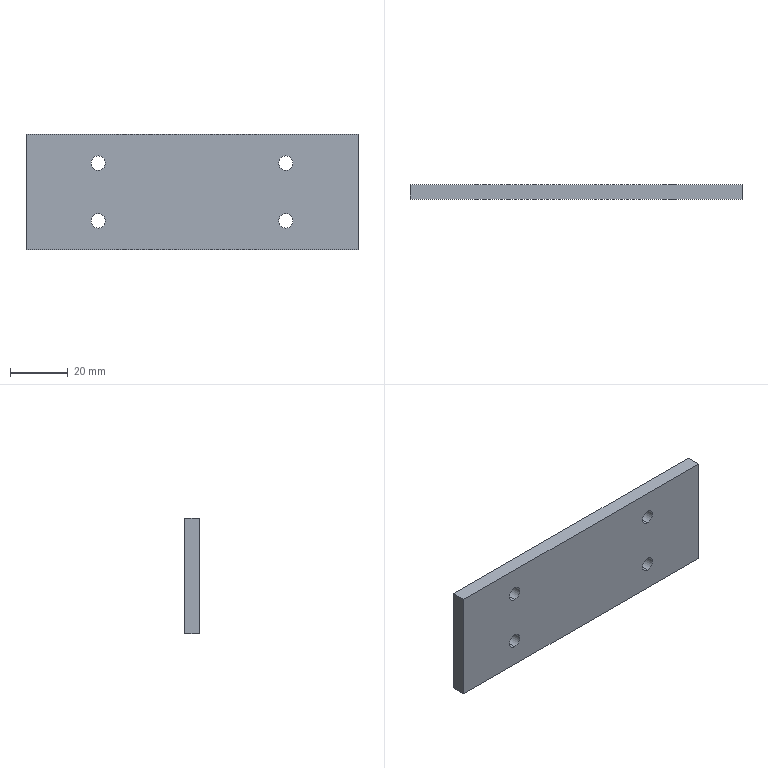Part | SolidWorks | features Extrusion 1, ICE 1 | 1 solid | 14 faces | box 115 x 5 x 40 mm | volume 22607 mm3 | cylinder 8 | plane 6 | commonest cylinder face diameters 5 x8
STEP:
#1=CARTESIAN_POINT('',(1.28,-0.09843,-0.2953));
#2=VERTEX_POINT('',#1);
#3=CARTESIAN_POINT('',(1.28,-0.09843,-0.4921));
#4=VERTEX_POINT('',#3);
#5=CARTESIAN_POINT('',(1.28,-0.09843,-0.3937));
#6=DIRECTION('',(0.,-1.,0.));
#7=DIRECTION('',(0.,0.,-1.));
#8=AXIS2_PLACEMENT_3D('',#5,#6,#7);
#9=CIRCLE('',#8,0.09843);
#10=EDGE_CURVE('',#2,#4,#9,.T.);
#11=ORIENTED_EDGE('',*,*,#10,.T.);
#12=CARTESIAN_POINT('',(1.28,0.09843,-0.4921));
#13=VERTEX_POINT('',#12);
#14=CARTESIAN_POINT('',(1.28,-1.476,-0.4921));
#15=DIRECTION('',(0.,1.,0.));
#16=VECTOR('',#15,39.37);
#17=LINE('',#14,#16);
#18=EDGE_CURVE('',#4,#13,#17,.T.);
#19=ORIENTED_EDGE('',*,*,#18,.T.);
#20=CARTESIAN_POINT('',(1.28,0.09843,-0.2953));
#21=VERTEX_POINT('',#20);
#22=CARTESIAN_POINT('',(1.28,0.09843,-0.3937));
#23=DIRECTION('',(0.,1.,0.));
#24=DIRECTION('',(0.,0.,1.));
#25=AXIS2_PLACEMENT_3D('',#22,#23,#24);
#26=CIRCLE('',#25,0.09843);
#27=EDGE_CURVE('',#13,#21,#26,.T.);
#28=ORIENTED_EDGE('',*,*,#27,.T.);
#29=CARTESIAN_POINT('',(1.28,-1.476,-0.2953));
#30=DIRECTION('',(0.,1.,0.));
#31=VECTOR('',#30,39.37);
#32=LINE('',#29,#31);
#33=EDGE_CURVE('',#2,#21,#32,.T.);
#34=ORIENTED_EDGE('',*,*,#33,.F.);
#35=EDGE_LOOP('',(#11,#19,#28,#34));
#36=FACE_OUTER_BOUND('',#35,.T.);
#37=CARTESIAN_POINT('',(1.28,-1.476,-0.3937));
#38=DIRECTION('',(0.,1.,0.));
#39=DIRECTION('',(0.,0.,1.));
#40=AXIS2_PLACEMENT_3D('',#37,#38,#39);
#41=CYLINDRICAL_SURFACE('',#40,0.09843);
#42=ADVANCED_FACE('',(#36),#41,.F.);
#43=CARTESIAN_POINT('',(-1.28,-0.09843,-0.2953));
#44=VERTEX_POINT('',#43);
#45=CARTESIAN_POINT('',(-1.28,-0.09843,-0.4921));
#46=VERTEX_POINT('',#45);
#47=CARTESIAN_POINT('',(-1.28,-0.09843,-0.3937));
#48=DIRECTION('',(0.,-1.,0.));
#49=DIRECTION('',(0.,0.,-1.));
#50=AXIS2_PLACEMENT_3D('',#47,#48,#49);
#51=CIRCLE('',#50,0.09843);
#52=EDGE_CURVE('',#44,#46,#51,.T.);
#53=ORIENTED_EDGE('',*,*,#52,.T.);
#54=CARTESIAN_POINT('',(-1.28,0.09843,-0.4921));
#55=VERTEX_POINT('',#54);
#56=CARTESIAN_POINT('',(-1.28,-1.476,-0.4921));
#57=DIRECTION('',(0.,1.,0.));
#58=VECTOR('',#57,39.37);
#59=LINE('',#56,#58);
#60=EDGE_CURVE('',#46,#55,#59,.T.);
#61=ORIENTED_EDGE('',*,*,#60,.T.);
#62=CARTESIAN_POINT('',(-1.28,0.09843,-0.2953));
#63=VERTEX_POINT('',#62);
#64=CARTESIAN_POINT('',(-1.28,0.09843,-0.3937));
#65=DIRECTION('',(0.,1.,0.));
#66=DIRECTION('',(0.,0.,1.));
#67=AXIS2_PLACEMENT_3D('',#64,#65,#66);
#68=CIRCLE('',#67,0.09843);
#69=EDGE_CURVE('',#55,#63,#68,.T.);
#70=ORIENTED_EDGE('',*,*,#69,.T.);
#71=CARTESIAN_POINT('',(-1.28,-1.476,-0.2953));
#72=DIRECTION('',(0.,1.,0.));
#73=VECTOR('',#72,39.37);
#74=LINE('',#71,#73);
#75=EDGE_CURVE('',#44,#63,#74,.T.);
#76=ORIENTED_EDGE('',*,*,#75,.F.);
#77=EDGE_LOOP('',(#53,#61,#70,#76));
#78=FACE_OUTER_BOUND('',#77,.T.);
#79=CARTESIAN_POINT('',(-1.28,-1.476,-0.3937));
#80=DIRECTION('',(0.,1.,0.));
#81=DIRECTION('',(0.,0.,1.));
#82=AXIS2_PLACEMENT_3D('',#79,#80,#81);
#83=CYLINDRICAL_SURFACE('',#82,0.09843);
#84=ADVANCED_FACE('',(#78),#83,.F.);
#85=CARTESIAN_POINT('',(1.28,-0.09843,-1.083));
#86=VERTEX_POINT('',#85);
#87=CARTESIAN_POINT('',(1.28,-0.09843,-1.28));
#88=VERTEX_POINT('',#87);
#89=CARTESIAN_POINT('',(1.28,-0.09843,-1.181));
#90=DIRECTION('',(0.,-1.,0.));
#91=DIRECTION('',(0.,0.,-1.));
#92=AXIS2_PLACEMENT_3D('',#89,#90,#91);
#93=CIRCLE('',#92,0.09843);
#94=EDGE_CURVE('',#86,#88,#93,.T.);
#95=ORIENTED_EDGE('',*,*,#94,.T.);
#96=CARTESIAN_POINT('',(1.28,0.09843,-1.28));
#97=VERTEX_POINT('',#96);
#98=CARTESIAN_POINT('',(1.28,-1.476,-1.28));
#99=DIRECTION('',(0.,1.,0.));
#100=VECTOR('',#99,39.37);
#101=LINE('',#98,#100);
#102=EDGE_CURVE('',#88,#97,#101,.T.);
#103=ORIENTED_EDGE('',*,*,#102,.T.);
#104=CARTESIAN_POINT('',(1.28,0.09843,-1.083));
#105=VERTEX_POINT('',#104);
#106=CARTESIAN_POINT('',(1.28,0.09843,-1.181));
#107=DIRECTION('',(0.,1.,0.));
#108=DIRECTION('',(0.,0.,1.));
#109=AXIS2_PLACEMENT_3D('',#106,#107,#108);
#110=CIRCLE('',#109,0.09843);
#111=EDGE_CURVE('',#97,#105,#110,.T.);
#112=ORIENTED_EDGE('',*,*,#111,.T.);
#113=CARTESIAN_POINT('',(1.28,-1.476,-1.083));
#114=DIRECTION('',(0.,1.,0.));
#115=VECTOR('',#114,39.37);
#116=LINE('',#113,#115);
#117=EDGE_CURVE('',#86,#105,#116,.T.);
#118=ORIENTED_EDGE('',*,*,#117,.F.);
#119=EDGE_LOOP('',(#95,#103,#112,#118));
#120=FACE_OUTER_BOUND('',#119,.T.);
#121=CARTESIAN_POINT('',(1.28,-1.476,-1.181));
#122=DIRECTION('',(0.,1.,0.));
#123=DIRECTION('',(0.,0.,1.));
#124=AXIS2_PLACEMENT_3D('',#121,#122,#123);
#125=CYLINDRICAL_SURFACE('',#124,0.09843);
#126=ADVANCED_FACE('',(#120),#125,.F.);
#127=CARTESIAN_POINT('',(-1.28,-0.09843,-1.083));
#128=VERTEX_POINT('',#127);
#129=CARTESIAN_POINT('',(-1.28,-0.09843,-1.28));
#130=VERTEX_POINT('',#129);
#131=CARTESIAN_POINT('',(-1.28,-0.09843,-1.181));
#132=DIRECTION('',(0.,-1.,0.));
#133=DIRECTION('',(0.,0.,-1.));
#134=AXIS2_PLACEMENT_3D('',#131,#132,#133);
#135=CIRCLE('',#134,0.09843);
#136=EDGE_CURVE('',#128,#130,#135,.T.);
#137=ORIENTED_EDGE('',*,*,#136,.T.);
#138=CARTESIAN_POINT('',(-1.28,0.09843,-1.28));
#139=VERTEX_POINT('',#138);
#140=CARTESIAN_POINT('',(-1.28,-1.476,-1.28));
#141=DIRECTION('',(0.,1.,0.));
#142=VECTOR('',#141,39.37);
#143=LINE('',#140,#142);
#144=EDGE_CURVE('',#130,#139,#143,.T.);
#145=ORIENTED_EDGE('',*,*,#144,.T.);
#146=CARTESIAN_POINT('',(-1.28,0.09843,-1.083));
#147=VERTEX_POINT('',#146);
#148=CARTESIAN_POINT('',(-1.28,0.09843,-1.181));
#149=DIRECTION('',(0.,1.,0.));
#150=DIRECTION('',(0.,0.,1.));
#151=AXIS2_PLACEMENT_3D('',#148,#149,#150);
#152=CIRCLE('',#151,0.09843);
#153=EDGE_CURVE('',#139,#147,#152,.T.);
#154=ORIENTED_EDGE('',*,*,#153,.T.);
#155=CARTESIAN_POINT('',(-1.28,-1.476,-1.083));
#156=DIRECTION('',(0.,1.,0.));
#157=VECTOR('',#156,39.37);
#158=LINE('',#155,#157);
#159=EDGE_CURVE('',#128,#147,#158,.T.);
#160=ORIENTED_EDGE('',*,*,#159,.F.);
#161=EDGE_LOOP('',(#137,#145,#154,#160));
#162=FACE_OUTER_BOUND('',#161,.T.);
#163=CARTESIAN_POINT('',(-1.28,-1.476,-1.181));
#164=DIRECTION('',(0.,1.,0.));
#165=DIRECTION('',(0.,0.,1.));
#166=AXIS2_PLACEMENT_3D('',#163,#164,#165);
#167=CYLINDRICAL_SURFACE('',#166,0.09843);
#168=ADVANCED_FACE('',(#162),#167,.F.);
#169=CARTESIAN_POINT('',(2.264,-0.09843,0.));
#170=VERTEX_POINT('',#169);
#171=CARTESIAN_POINT('',(2.264,0.09843,0.));
#172=VERTEX_POINT('',#171);
#173=CARTESIAN_POINT('',(2.264,0.09843,0.));
#174=DIRECTION('',(0.,1.,0.));
#175=VECTOR('',#174,39.37);
#176=LINE('',#173,#175);
#177=EDGE_CURVE('',#170,#172,#176,.T.);
#178=ORIENTED_EDGE('',*,*,#177,.F.);
#179=CARTESIAN_POINT('',(2.264,-0.09843,-1.575));
#180=VERTEX_POINT('',#179);
#181=CARTESIAN_POINT('',(2.264,-0.09843,-1.575));
#182=DIRECTION('',(0.,0.,1.));
#183=VECTOR('',#182,39.37);
#184=LINE('',#181,#183);
#185=EDGE_CURVE('',#180,#170,#184,.T.);
#186=ORIENTED_EDGE('',*,*,#185,.F.);
#187=CARTESIAN_POINT('',(2.264,0.09843,-1.575));
#188=VERTEX_POINT('',#187);
#189=CARTESIAN_POINT('',(2.264,0.09843,-1.575));
#190=DIRECTION('',(0.,1.,0.));
#191=VECTOR('',#190,39.37);
#192=LINE('',#189,#191);
#193=EDGE_CURVE('',#180,#188,#192,.T.);
#194=ORIENTED_EDGE('',*,*,#193,.T.);
#195=CARTESIAN_POINT('',(2.264,0.09843,-1.575));
#196=DIRECTION('',(0.,0.,1.));
#197=VECTOR('',#196,39.37);
#198=LINE('',#195,#197);
#199=EDGE_CURVE('',#188,#172,#198,.T.);
#200=ORIENTED_EDGE('',*,*,#199,.T.);
#201=EDGE_LOOP('',(#178,#186,#194,#200));
#202=FACE_OUTER_BOUND('',#201,.T.);
#203=CARTESIAN_POINT('',(2.264,0.09843,-1.575));
#204=DIRECTION('',(1.,0.,0.));
#205=DIRECTION('',(0.,0.,-1.));
#206=AXIS2_PLACEMENT_3D('',#203,#204,#205);
#207=PLANE('',#206);
#208=ADVANCED_FACE('',(#202),#207,.T.);
#209=ORIENTED_EDGE('',*,*,#10,.F.);
#210=CARTESIAN_POINT('',(1.28,-0.09843,-0.3937));
#211=DIRECTION('',(0.,-1.,0.));
#212=DIRECTION('',(0.,0.,-1.));
#213=AXIS2_PLACEMENT_3D('',#210,#211,#212);
#214=CIRCLE('',#213,0.09843);
#215=EDGE_CURVE('',#4,#2,#214,.T.);
#216=ORIENTED_EDGE('',*,*,#215,.F.);
#217=EDGE_LOOP('',(#209,#216));
#218=FACE_BOUND('',#217,.T.);
#219=ORIENTED_EDGE('',*,*,#52,.F.);
#220=CARTESIAN_POINT('',(-1.28,-0.09843,-0.3937));
#221=DIRECTION('',(0.,-1.,0.));
#222=DIRECTION('',(0.,0.,-1.));
#223=AXIS2_PLACEMENT_3D('',#220,#221,#222);
#224=CIRCLE('',#223,0.09843);
#225=EDGE_CURVE('',#46,#44,#224,.T.);
#226=ORIENTED_EDGE('',*,*,#225,.F.);
#227=EDGE_LOOP('',(#219,#226));
#228=FACE_BOUND('',#227,.T.);
#229=ORIENTED_EDGE('',*,*,#94,.F.);
#230=CARTESIAN_POINT('',(1.28,-0.09843,-1.181));
#231=DIRECTION('',(0.,-1.,0.));
#232=DIRECTION('',(0.,0.,-1.));
#233=AXIS2_PLACEMENT_3D('',#230,#231,#232);
#234=CIRCLE('',#233,0.09843);
#235=EDGE_CURVE('',#88,#86,#234,.T.);
#236=ORIENTED_EDGE('',*,*,#235,.F.);
#237=EDGE_LOOP('',(#229,#236));
#238=FACE_BOUND('',#237,.T.);
#239=ORIENTED_EDGE('',*,*,#136,.F.);
#240=CARTESIAN_POINT('',(-1.28,-0.09843,-1.181));
#241=DIRECTION('',(0.,-1.,0.));
#242=DIRECTION('',(0.,0.,-1.));
#243=AXIS2_PLACEMENT_3D('',#240,#241,#242);
#244=CIRCLE('',#243,0.09843);
#245=EDGE_CURVE('',#130,#128,#244,.T.);
#246=ORIENTED_EDGE('',*,*,#245,.F.);
#247=EDGE_LOOP('',(#239,#246));
#248=FACE_BOUND('',#247,.T.);
#249=CARTESIAN_POINT('',(-2.264,-0.09843,0.));
#250=VERTEX_POINT('',#249);
#251=CARTESIAN_POINT('',(-2.264,-0.09843,0.));
#252=DIRECTION('',(1.,0.,0.));
#253=VECTOR('',#252,39.37);
#254=LINE('',#251,#253);
#255=EDGE_CURVE('',#250,#170,#254,.T.);
#256=ORIENTED_EDGE('',*,*,#255,.F.);
#257=CARTESIAN_POINT('',(-2.264,-0.09843,-1.575));
#258=VERTEX_POINT('',#257);
#259=CARTESIAN_POINT('',(-2.264,-0.09843,-1.575));
#260=DIRECTION('',(0.,0.,1.));
#261=VECTOR('',#260,39.37);
#262=LINE('',#259,#261);
#263=EDGE_CURVE('',#258,#250,#262,.T.);
#264=ORIENTED_EDGE('',*,*,#263,.F.);
#265=CARTESIAN_POINT('',(-2.264,-0.09843,-1.575));
#266=DIRECTION('',(1.,0.,0.));
#267=VECTOR('',#266,39.37);
#268=LINE('',#265,#267);
#269=EDGE_CURVE('',#258,#180,#268,.T.);
#270=ORIENTED_EDGE('',*,*,#269,.T.);
#271=ORIENTED_EDGE('',*,*,#185,.T.);
#272=EDGE_LOOP('',(#256,#264,#270,#271));
#273=FACE_OUTER_BOUND('',#272,.T.);
#274=CARTESIAN_POINT('',(-2.264,-0.09843,-1.575));
#275=DIRECTION('',(0.,-1.,0.));
#276=DIRECTION('',(0.,0.,-1.));
#277=AXIS2_PLACEMENT_3D('',#274,#275,#276);
#278=PLANE('',#277);
#279=ADVANCED_FACE('',(#218,#228,#238,#248,#273),#278,.T.);
#280=CARTESIAN_POINT('',(-2.264,0.09843,0.));
#281=VERTEX_POINT('',#280);
#282=CARTESIAN_POINT('',(-2.264,0.09843,0.));
#283=DIRECTION('',(0.,-1.,0.));
#284=VECTOR('',#283,39.37);
#285=LINE('',#282,#284);
#286=EDGE_CURVE('',#281,#250,#285,.T.);
#287=ORIENTED_EDGE('',*,*,#286,.F.);
#288=CARTESIAN_POINT('',(-2.264,0.09843,-1.575));
#289=VERTEX_POINT('',#288);
#290=CARTESIAN_POINT('',(-2.264,0.09843,-1.575));
#291=DIRECTION('',(0.,0.,1.));
#292=VECTOR('',#291,39.37);
#293=LINE('',#290,#292);
#294=EDGE_CURVE('',#289,#281,#293,.T.);
#295=ORIENTED_EDGE('',*,*,#294,.F.);
#296=CARTESIAN_POINT('',(-2.264,0.09843,-1.575));
#297=DIRECTION('',(0.,-1.,0.));
#298=VECTOR('',#297,39.37);
#299=LINE('',#296,#298);
#300=EDGE_CURVE('',#289,#258,#299,.T.);
#301=ORIENTED_EDGE('',*,*,#300,.T.);
#302=ORIENTED_EDGE('',*,*,#263,.T.);
#303=EDGE_LOOP('',(#287,#295,#301,#302));
#304=FACE_OUTER_BOUND('',#303,.T.);
#305=CARTESIAN_POINT('',(-2.264,0.09843,-1.575));
#306=DIRECTION('',(-1.,0.,0.));
#307=DIRECTION('',(0.,0.,1.));
#308=AXIS2_PLACEMENT_3D('',#305,#306,#307);
#309=PLANE('',#308);
#310=ADVANCED_FACE('',(#304),#309,.T.);
#311=CARTESIAN_POINT('',(1.28,0.09843,-0.3937));
#312=DIRECTION('',(0.,1.,0.));
#313=DIRECTION('',(0.,0.,1.));
#314=AXIS2_PLACEMENT_3D('',#311,#312,#313);
#315=CIRCLE('',#314,0.09843);
#316=EDGE_CURVE('',#21,#13,#315,.T.);
#317=ORIENTED_EDGE('',*,*,#316,.F.);
#318=ORIENTED_EDGE('',*,*,#27,.F.);
#319=EDGE_LOOP('',(#317,#318));
#320=FACE_BOUND('',#319,.T.);
#321=CARTESIAN_POINT('',(-1.28,0.09843,-0.3937));
#322=DIRECTION('',(0.,1.,0.));
#323=DIRECTION('',(0.,0.,1.));
#324=AXIS2_PLACEMENT_3D('',#321,#322,#323);
#325=CIRCLE('',#324,0.09843);
#326=EDGE_CURVE('',#63,#55,#325,.T.);
#327=ORIENTED_EDGE('',*,*,#326,.F.);
#328=ORIENTED_EDGE('',*,*,#69,.F.);
#329=EDGE_LOOP('',(#327,#328));
#330=FACE_BOUND('',#329,.T.);
#331=CARTESIAN_POINT('',(1.28,0.09843,-1.181));
#332=DIRECTION('',(0.,1.,0.));
#333=DIRECTION('',(0.,0.,1.));
#334=AXIS2_PLACEMENT_3D('',#331,#332,#333);
#335=CIRCLE('',#334,0.09843);
#336=EDGE_CURVE('',#105,#97,#335,.T.);
#337=ORIENTED_EDGE('',*,*,#336,.F.);
#338=ORIENTED_EDGE('',*,*,#111,.F.);
#339=EDGE_LOOP('',(#337,#338));
#340=FACE_BOUND('',#339,.T.);
#341=CARTESIAN_POINT('',(-1.28,0.09843,-1.181));
#342=DIRECTION('',(0.,1.,0.));
#343=DIRECTION('',(0.,0.,1.));
#344=AXIS2_PLACEMENT_3D('',#341,#342,#343);
#345=CIRCLE('',#344,0.09843);
#346=EDGE_CURVE('',#147,#139,#345,.T.);
#347=ORIENTED_EDGE('',*,*,#346,.F.);
#348=ORIENTED_EDGE('',*,*,#153,.F.);
#349=EDGE_LOOP('',(#347,#348));
#350=FACE_BOUND('',#349,.T.);
#351=CARTESIAN_POINT('',(-2.264,0.09843,0.));
#352=DIRECTION('',(-1.,0.,0.));
#353=VECTOR('',#352,39.37);
#354=LINE('',#351,#353);
#355=EDGE_CURVE('',#172,#281,#354,.T.);
#356=ORIENTED_EDGE('',*,*,#355,.F.);
#357=ORIENTED_EDGE('',*,*,#199,.F.);
#358=CARTESIAN_POINT('',(-2.264,0.09843,-1.575));
#359=DIRECTION('',(-1.,0.,0.));
#360=VECTOR('',#359,39.37);
#361=LINE('',#358,#360);
#362=EDGE_CURVE('',#188,#289,#361,.T.);
#363=ORIENTED_EDGE('',*,*,#362,.T.);
#364=ORIENTED_EDGE('',*,*,#294,.T.);
#365=EDGE_LOOP('',(#356,#357,#363,#364));
#366=FACE_OUTER_BOUND('',#365,.T.);
#367=CARTESIAN_POINT('',(-2.264,0.09843,-1.575));
#368=DIRECTION('',(0.,1.,0.));
#369=DIRECTION('',(0.,0.,1.));
#370=AXIS2_PLACEMENT_3D('',#367,#368,#369);
#371=PLANE('',#370);
#372=ADVANCED_FACE('',(#320,#330,#340,#350,#366),#371,.T.);
#373=ORIENTED_EDGE('',*,*,#193,.F.);
#374=ORIENTED_EDGE('',*,*,#269,.F.);
#375=ORIENTED_EDGE('',*,*,#300,.F.);
#376=ORIENTED_EDGE('',*,*,#362,.F.);
#377=EDGE_LOOP('',(#373,#374,#375,#376));
#378=FACE_OUTER_BOUND('',#377,.T.);
#379=CARTESIAN_POINT('',(0.,0.,-1.575));
#380=DIRECTION('',(0.,0.,1.));
#381=DIRECTION('',(1.,0.,0.));
#382=AXIS2_PLACEMENT_3D('',#379,#380,#381);
#383=PLANE('',#382);
#384=ADVANCED_FACE('',(#378),#383,.F.);
#385=ORIENTED_EDGE('',*,*,#177,.T.);
#386=ORIENTED_EDGE('',*,*,#355,.T.);
#387=ORIENTED_EDGE('',*,*,#286,.T.);
#388=ORIENTED_EDGE('',*,*,#255,.T.);
#389=EDGE_LOOP('',(#385,#386,#387,#388));
#390=FACE_OUTER_BOUND('',#389,.T.);
#391=CARTESIAN_POINT('',(0.,0.,0.));
#392=DIRECTION('',(0.,0.,1.));
#393=DIRECTION('',(1.,0.,0.));
#394=AXIS2_PLACEMENT_3D('',#391,#392,#393);
#395=PLANE('',#394);
#396=ADVANCED_FACE('',(#390),#395,.T.);
#397=ORIENTED_EDGE('',*,*,#144,.F.);
#398=ORIENTED_EDGE('',*,*,#245,.T.);
#399=ORIENTED_EDGE('',*,*,#159,.T.);
#400=ORIENTED_EDGE('',*,*,#346,.T.);
#401=EDGE_LOOP('',(#397,#398,#399,#400));
#402=FACE_OUTER_BOUND('',#401,.T.);
#403=CARTESIAN_POINT('',(-1.28,-1.476,-1.181));
#404=DIRECTION('',(0.,1.,0.));
#405=DIRECTION('',(0.,0.,1.));
#406=AXIS2_PLACEMENT_3D('',#403,#404,#405);
#407=CYLINDRICAL_SURFACE('',#406,0.09843);
#408=ADVANCED_FACE('',(#402),#407,.F.);
#409=ORIENTED_EDGE('',*,*,#102,.F.);
#410=ORIENTED_EDGE('',*,*,#235,.T.);
#411=ORIENTED_EDGE('',*,*,#117,.T.);
#412=ORIENTED_EDGE('',*,*,#336,.T.);
#413=EDGE_LOOP('',(#409,#410,#411,#412));
#414=FACE_OUTER_BOUND('',#413,.T.);
#415=CARTESIAN_POINT('',(1.28,-1.476,-1.181));
#416=DIRECTION('',(0.,1.,0.));
#417=DIRECTION('',(0.,0.,1.));
#418=AXIS2_PLACEMENT_3D('',#415,#416,#417);
#419=CYLINDRICAL_SURFACE('',#418,0.09843);
#420=ADVANCED_FACE('',(#414),#419,.F.);
#421=ORIENTED_EDGE('',*,*,#60,.F.);
#422=ORIENTED_EDGE('',*,*,#225,.T.);
#423=ORIENTED_EDGE('',*,*,#75,.T.);
#424=ORIENTED_EDGE('',*,*,#326,.T.);
#425=EDGE_LOOP('',(#421,#422,#423,#424));
#426=FACE_OUTER_BOUND('',#425,.T.);
#427=CARTESIAN_POINT('',(-1.28,-1.476,-0.3937));
#428=DIRECTION('',(0.,1.,0.));
#429=DIRECTION('',(0.,0.,1.));
#430=AXIS2_PLACEMENT_3D('',#427,#428,#429);
#431=CYLINDRICAL_SURFACE('',#430,0.09843);
#432=ADVANCED_FACE('',(#426),#431,.F.);
#433=ORIENTED_EDGE('',*,*,#18,.F.);
#434=ORIENTED_EDGE('',*,*,#215,.T.);
#435=ORIENTED_EDGE('',*,*,#33,.T.);
#436=ORIENTED_EDGE('',*,*,#316,.T.);
#437=EDGE_LOOP('',(#433,#434,#435,#436));
#438=FACE_OUTER_BOUND('',#437,.T.);
#439=CARTESIAN_POINT('',(1.28,-1.476,-0.3937));
#440=DIRECTION('',(0.,1.,0.));
#441=DIRECTION('',(0.,0.,1.));
#442=AXIS2_PLACEMENT_3D('',#439,#440,#441);
#443=CYLINDRICAL_SURFACE('',#442,0.09843);
#444=ADVANCED_FACE('',(#438),#443,.F.);
#445=CLOSED_SHELL('',(#42,#84,#126,#168,#208,#279,#310,#372,#384,#396,#408,#420,#432,#444));
#446=MANIFOLD_SOLID_BREP('',#445);
#447=CARTESIAN_POINT('',(0.,0.,0.));
#448=DIRECTION('',(0.,0.,1.));
#449=DIRECTION('',(1.,0.,0.));
#450=AXIS2_PLACEMENT_3D('',#447,#448,#449);
#451=(LENGTH_UNIT()NAMED_UNIT(*)SI_UNIT($,.METRE.));
#452=LENGTH_MEASURE_WITH_UNIT(LENGTH_MEASURE(0.0254),#451);
#453=DIMENSIONAL_EXPONENTS(1.,0.,0.,0.,0.,0.,0.);
#454=(CONVERSION_BASED_UNIT('INCH',#452)LENGTH_UNIT()NAMED_UNIT(#453));
#455=UNCERTAINTY_MEASURE_WITH_UNIT(LENGTH_MEASURE(0.00001),#454,'','');
#456=(NAMED_UNIT(*)PLANE_ANGLE_UNIT()SI_UNIT($,.RADIAN.));
#457=(NAMED_UNIT(*)SI_UNIT($,.STERADIAN.)SOLID_ANGLE_UNIT());
#458=(GEOMETRIC_REPRESENTATION_CONTEXT(3)GLOBAL_UNCERTAINTY_ASSIGNED_CONTEXT((#455))GLOBAL_UNIT_ASSIGNED_CONTEXT((#454,#456,#457))REPRESENTATION_CONTEXT('',''));
#459=ADVANCED_BREP_SHAPE_REPRESENTATION('',(#446,#450),#458);